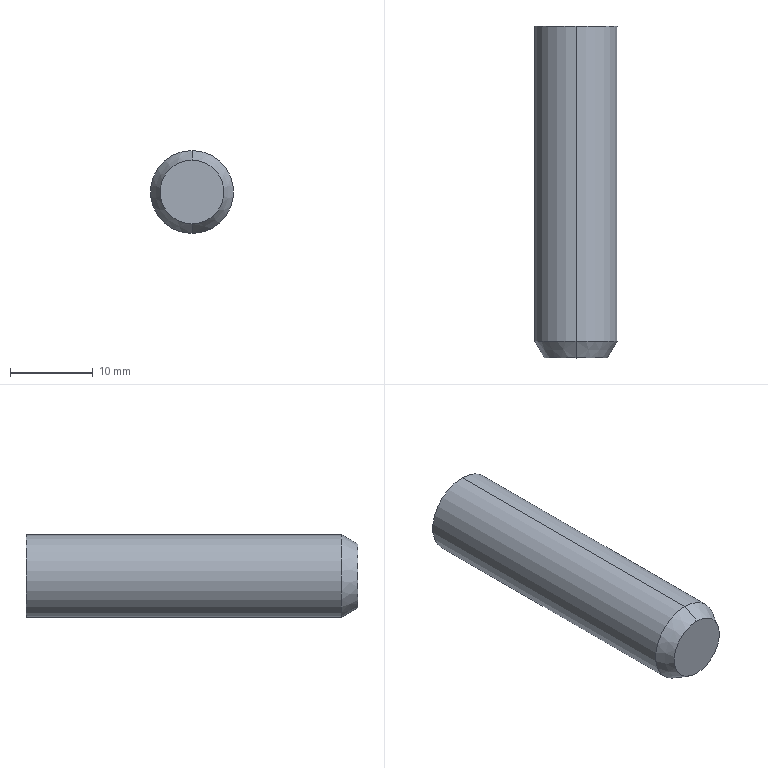Part | SolidWorks | features Chamfer 1, Extrusion 1 | 1 solid | 6 faces | box 10 x 40 x 10 mm | volume 3108 mm3 | cone 2 | cylinder 2 | plane 2 | commonest cylinder face diameters 10 x2
STEP:
#1=CARTESIAN_POINT('',(0.,0.,-3.845));
#2=VERTEX_POINT('',#1);
#3=CARTESIAN_POINT('',(0.,0.,3.845));
#4=VERTEX_POINT('',#3);
#5=CARTESIAN_POINT('',(0.,0.,0.));
#6=DIRECTION('',(0.,-1.,0.));
#7=DIRECTION('',(0.,0.,1.));
#8=AXIS2_PLACEMENT_3D('',#5,#6,#7);
#9=CIRCLE('',#8,3.845);
#10=EDGE_CURVE('',#2,#4,#9,.T.);
#11=ORIENTED_EDGE('',*,*,#10,.F.);
#12=CARTESIAN_POINT('',(0.,2.,-5.));
#13=VERTEX_POINT('',#12);
#14=CARTESIAN_POINT('',(0.,2.,-5.));
#15=DIRECTION('',(0.,0.866,-0.5));
#16=VECTOR('',#15,1000.);
#17=LINE('',#14,#16);
#18=EDGE_CURVE('',#2,#13,#17,.T.);
#19=ORIENTED_EDGE('',*,*,#18,.T.);
#20=CARTESIAN_POINT('',(0.,2.,5.));
#21=VERTEX_POINT('',#20);
#22=CARTESIAN_POINT('',(0.,2.,0.));
#23=DIRECTION('',(0.,1.,0.));
#24=DIRECTION('',(0.,0.,1.));
#25=AXIS2_PLACEMENT_3D('',#22,#23,#24);
#26=CIRCLE('',#25,5.);
#27=EDGE_CURVE('',#21,#13,#26,.T.);
#28=ORIENTED_EDGE('',*,*,#27,.F.);
#29=CARTESIAN_POINT('',(0.,2.,5.));
#30=DIRECTION('',(0.,0.866,0.5));
#31=VECTOR('',#30,1000.);
#32=LINE('',#29,#31);
#33=EDGE_CURVE('',#4,#21,#32,.T.);
#34=ORIENTED_EDGE('',*,*,#33,.F.);
#35=EDGE_LOOP('',(#11,#19,#28,#34));
#36=FACE_OUTER_BOUND('',#35,.T.);
#37=CARTESIAN_POINT('',(0.,2.,0.));
#38=DIRECTION('',(0.,1.,0.));
#39=DIRECTION('',(0.,0.,1.));
#40=AXIS2_PLACEMENT_3D('',#37,#38,#39);
#41=CONICAL_SURFACE('',#40,5.,0.5236);
#42=ADVANCED_FACE('',(#36),#41,.T.);
#43=CARTESIAN_POINT('',(0.,40.,5.));
#44=VERTEX_POINT('',#43);
#45=CARTESIAN_POINT('',(0.,40.,-5.));
#46=VERTEX_POINT('',#45);
#47=CARTESIAN_POINT('',(0.,40.,0.));
#48=DIRECTION('',(0.,1.,0.));
#49=DIRECTION('',(0.,0.,1.));
#50=AXIS2_PLACEMENT_3D('',#47,#48,#49);
#51=CIRCLE('',#50,5.);
#52=EDGE_CURVE('',#44,#46,#51,.T.);
#53=ORIENTED_EDGE('',*,*,#52,.F.);
#54=CARTESIAN_POINT('',(0.,40.,5.));
#55=DIRECTION('',(0.,-1.,0.));
#56=VECTOR('',#55,1000.);
#57=LINE('',#54,#56);
#58=EDGE_CURVE('',#44,#21,#57,.T.);
#59=ORIENTED_EDGE('',*,*,#58,.T.);
#60=ORIENTED_EDGE('',*,*,#27,.T.);
#61=CARTESIAN_POINT('',(0.,40.,-5.));
#62=DIRECTION('',(0.,-1.,0.));
#63=VECTOR('',#62,1000.);
#64=LINE('',#61,#63);
#65=EDGE_CURVE('',#46,#13,#64,.T.);
#66=ORIENTED_EDGE('',*,*,#65,.F.);
#67=EDGE_LOOP('',(#53,#59,#60,#66));
#68=FACE_OUTER_BOUND('',#67,.T.);
#69=CARTESIAN_POINT('',(0.,40.,0.));
#70=DIRECTION('',(0.,-1.,0.));
#71=DIRECTION('',(0.,0.,-1.));
#72=AXIS2_PLACEMENT_3D('',#69,#70,#71);
#73=CYLINDRICAL_SURFACE('',#72,5.);
#74=ADVANCED_FACE('',(#68),#73,.T.);
#75=ORIENTED_EDGE('',*,*,#58,.F.);
#76=CARTESIAN_POINT('',(0.,40.,0.));
#77=DIRECTION('',(0.,1.,0.));
#78=DIRECTION('',(0.,0.,1.));
#79=AXIS2_PLACEMENT_3D('',#76,#77,#78);
#80=CIRCLE('',#79,5.);
#81=EDGE_CURVE('',#46,#44,#80,.T.);
#82=ORIENTED_EDGE('',*,*,#81,.F.);
#83=ORIENTED_EDGE('',*,*,#65,.T.);
#84=CARTESIAN_POINT('',(0.,2.,0.));
#85=DIRECTION('',(0.,1.,0.));
#86=DIRECTION('',(0.,0.,1.));
#87=AXIS2_PLACEMENT_3D('',#84,#85,#86);
#88=CIRCLE('',#87,5.);
#89=EDGE_CURVE('',#13,#21,#88,.T.);
#90=ORIENTED_EDGE('',*,*,#89,.T.);
#91=EDGE_LOOP('',(#75,#82,#83,#90));
#92=FACE_OUTER_BOUND('',#91,.T.);
#93=CARTESIAN_POINT('',(0.,40.,0.));
#94=DIRECTION('',(0.,-1.,0.));
#95=DIRECTION('',(0.,0.,-1.));
#96=AXIS2_PLACEMENT_3D('',#93,#94,#95);
#97=CYLINDRICAL_SURFACE('',#96,5.);
#98=ADVANCED_FACE('',(#92),#97,.T.);
#99=ORIENTED_EDGE('',*,*,#81,.T.);
#100=ORIENTED_EDGE('',*,*,#52,.T.);
#101=EDGE_LOOP('',(#99,#100));
#102=FACE_OUTER_BOUND('',#101,.T.);
#103=CARTESIAN_POINT('',(0.,40.,0.));
#104=DIRECTION('',(0.,1.,0.));
#105=DIRECTION('',(0.,0.,1.));
#106=AXIS2_PLACEMENT_3D('',#103,#104,#105);
#107=PLANE('',#106);
#108=ADVANCED_FACE('',(#102),#107,.T.);
#109=CARTESIAN_POINT('',(0.,0.,0.));
#110=DIRECTION('',(0.,-1.,0.));
#111=DIRECTION('',(0.,0.,1.));
#112=AXIS2_PLACEMENT_3D('',#109,#110,#111);
#113=CIRCLE('',#112,3.845);
#114=EDGE_CURVE('',#4,#2,#113,.T.);
#115=ORIENTED_EDGE('',*,*,#114,.T.);
#116=ORIENTED_EDGE('',*,*,#10,.T.);
#117=EDGE_LOOP('',(#115,#116));
#118=FACE_OUTER_BOUND('',#117,.T.);
#119=CARTESIAN_POINT('',(0.,0.,0.));
#120=DIRECTION('',(0.,1.,0.));
#121=DIRECTION('',(0.,0.,1.));
#122=AXIS2_PLACEMENT_3D('',#119,#120,#121);
#123=PLANE('',#122);
#124=ADVANCED_FACE('',(#118),#123,.F.);
#125=ORIENTED_EDGE('',*,*,#18,.F.);
#126=ORIENTED_EDGE('',*,*,#114,.F.);
#127=ORIENTED_EDGE('',*,*,#33,.T.);
#128=ORIENTED_EDGE('',*,*,#89,.F.);
#129=EDGE_LOOP('',(#125,#126,#127,#128));
#130=FACE_OUTER_BOUND('',#129,.T.);
#131=CARTESIAN_POINT('',(0.,2.,0.));
#132=DIRECTION('',(0.,1.,0.));
#133=DIRECTION('',(0.,0.,1.));
#134=AXIS2_PLACEMENT_3D('',#131,#132,#133);
#135=CONICAL_SURFACE('',#134,5.,0.5236);
#136=ADVANCED_FACE('',(#130),#135,.T.);
#137=CLOSED_SHELL('',(#42,#74,#98,#108,#124,#136));
#138=MANIFOLD_SOLID_BREP('',#137);
#139=CARTESIAN_POINT('',(0.,0.,0.));
#140=DIRECTION('',(0.,0.,1.));
#141=DIRECTION('',(1.,0.,0.));
#142=AXIS2_PLACEMENT_3D('',#139,#140,#141);
#143=(LENGTH_UNIT()NAMED_UNIT(*)SI_UNIT(.MILLI.,.METRE.));
#144=UNCERTAINTY_MEASURE_WITH_UNIT(LENGTH_MEASURE(0.00001),#143,'','');
#145=(NAMED_UNIT(*)PLANE_ANGLE_UNIT()SI_UNIT($,.RADIAN.));
#146=(NAMED_UNIT(*)SI_UNIT($,.STERADIAN.)SOLID_ANGLE_UNIT());
#147=(GEOMETRIC_REPRESENTATION_CONTEXT(3)GLOBAL_UNCERTAINTY_ASSIGNED_CONTEXT((#144))GLOBAL_UNIT_ASSIGNED_CONTEXT((#143,#145,#146))REPRESENTATION_CONTEXT('',''));
#148=ADVANCED_BREP_SHAPE_REPRESENTATION('',(#138,#142),#147);